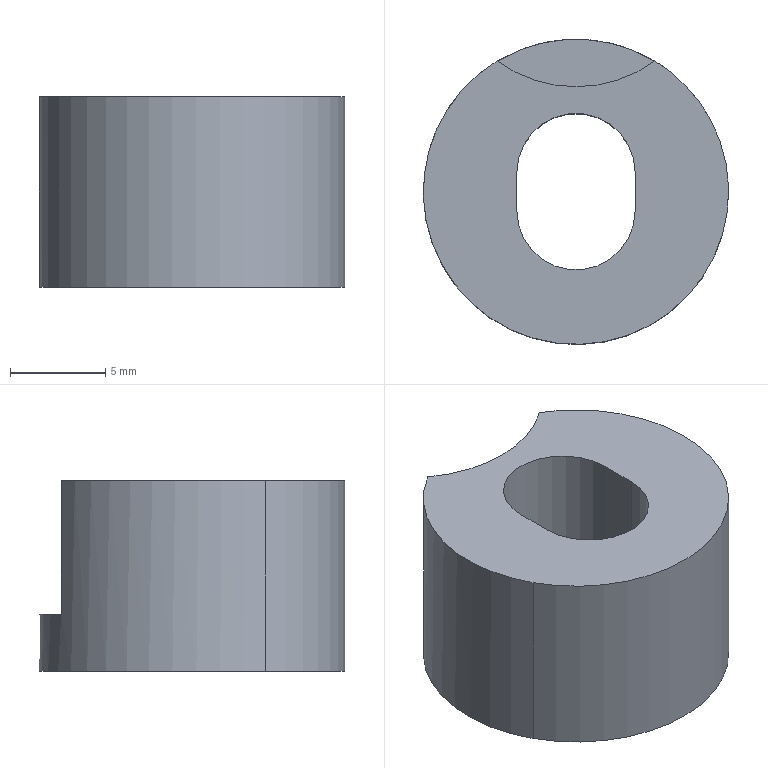Part | CATIA | 1 solid | 10 faces | box 16 x 16 x 10 mm | volume 1487 mm3 | cylinder 5 | plane 5 | commonest cylinder face diameters 6.2 x2 16 x2 14 x1
STEP:
#1=CARTESIAN_POINT('',(7.021,3.835,-10.));
#2=VERTEX_POINT('',#1);
#3=CARTESIAN_POINT('',(7.021,3.835,0.));
#4=VERTEX_POINT('',#3);
#5=CARTESIAN_POINT('',(7.021,3.835,-5.));
#6=DIRECTION('',(0.,0.,1.));
#7=VECTOR('',#6,1.);
#8=LINE('',#5,#7);
#9=EDGE_CURVE('',#2,#4,#8,.T.);
#10=ORIENTED_EDGE('',*,*,#9,.T.);
#11=CARTESIAN_POINT('',(-7.021,-3.835,0.));
#12=VERTEX_POINT('',#11);
#13=CARTESIAN_POINT('',(0.,0.,0.));
#14=DIRECTION('',(0.,0.,1.));
#15=AXIS2_PLACEMENT_3D('',#13,#14,$);
#16=CIRCLE('',#15,8.);
#17=EDGE_CURVE('',#12,#4,#16,.T.);
#18=ORIENTED_EDGE('',*,*,#17,.F.);
#19=CARTESIAN_POINT('',(-7.021,-3.835,-10.));
#20=VERTEX_POINT('',#19);
#21=CARTESIAN_POINT('',(-7.021,-3.835,-5.));
#22=DIRECTION('',(0.,0.,1.));
#23=VECTOR('',#22,1.);
#24=LINE('',#21,#23);
#25=EDGE_CURVE('',#20,#12,#24,.T.);
#26=ORIENTED_EDGE('',*,*,#25,.F.);
#27=CARTESIAN_POINT('',(0.,0.,-10.));
#28=DIRECTION('',(0.,0.,1.));
#29=AXIS2_PLACEMENT_3D('',#27,#28,$);
#30=CIRCLE('',#29,8.);
#31=EDGE_CURVE('',#20,#2,#30,.T.);
#32=ORIENTED_EDGE('',*,*,#31,.T.);
#33=EDGE_LOOP('',(#10,#18,#26,#32));
#34=FACE_OUTER_BOUND('',#33,.T.);
#35=CARTESIAN_POINT('',(0.,0.,-5.));
#36=DIRECTION('',(0.,0.,1.));
#37=DIRECTION('',(0.8776,0.4794,0.));
#38=AXIS2_PLACEMENT_3D('',#35,#36,#37);
#39=CYLINDRICAL_SURFACE('',#38,8.);
#40=ADVANCED_FACE('',(#34),#39,.T.);
#41=ORIENTED_EDGE('',*,*,#31,.F.);
#42=CARTESIAN_POINT('',(0.,0.,-10.));
#43=DIRECTION('',(0.,0.,1.));
#44=AXIS2_PLACEMENT_3D('',#42,#43,$);
#45=CIRCLE('',#44,8.);
#46=EDGE_CURVE('',#2,#20,#45,.T.);
#47=ORIENTED_EDGE('',*,*,#46,.F.);
#48=EDGE_LOOP('',(#41,#47));
#49=FACE_OUTER_BOUND('',#48,.T.);
#50=CARTESIAN_POINT('',(3.1,1.,-10.));
#51=VERTEX_POINT('',#50);
#52=CARTESIAN_POINT('',(-3.1,1.,-10.));
#53=VERTEX_POINT('',#52);
#54=CARTESIAN_POINT('',(0.,1.,-10.));
#55=DIRECTION('',(0.,0.,1.));
#56=AXIS2_PLACEMENT_3D('',#54,#55,$);
#57=CIRCLE('',#56,3.1);
#58=EDGE_CURVE('',#51,#53,#57,.T.);
#59=ORIENTED_EDGE('',*,*,#58,.T.);
#60=CARTESIAN_POINT('',(-3.1,-1.,-10.));
#61=VERTEX_POINT('',#60);
#62=CARTESIAN_POINT('',(-3.1,0.,-10.));
#63=DIRECTION('',(0.,1.,0.));
#64=VECTOR('',#63,1.);
#65=LINE('',#62,#64);
#66=EDGE_CURVE('',#61,#53,#65,.T.);
#67=ORIENTED_EDGE('',*,*,#66,.F.);
#68=CARTESIAN_POINT('',(3.1,-1.,-10.));
#69=VERTEX_POINT('',#68);
#70=CARTESIAN_POINT('',(0.,-1.,-10.));
#71=DIRECTION('',(0.,0.,1.));
#72=AXIS2_PLACEMENT_3D('',#70,#71,$);
#73=CIRCLE('',#72,3.1);
#74=EDGE_CURVE('',#61,#69,#73,.T.);
#75=ORIENTED_EDGE('',*,*,#74,.T.);
#76=CARTESIAN_POINT('',(3.1,0.,-10.));
#77=DIRECTION('',(0.,-1.,0.));
#78=VECTOR('',#77,1.);
#79=LINE('',#76,#78);
#80=EDGE_CURVE('',#51,#69,#79,.T.);
#81=ORIENTED_EDGE('',*,*,#80,.F.);
#82=EDGE_LOOP('',(#59,#67,#75,#81));
#83=FACE_BOUND('',#82,.T.);
#84=CARTESIAN_POINT('',(8.,0.,-10.));
#85=DIRECTION('',(0.,0.,1.));
#86=DIRECTION('',(1.,0.,0.));
#87=AXIS2_PLACEMENT_3D('',#84,#85,#86);
#88=PLANE('',#87);
#89=ADVANCED_FACE('',(#49,#83),#88,.F.);
#90=ORIENTED_EDGE('',*,*,#58,.F.);
#91=CARTESIAN_POINT('',(3.1,1.,0.));
#92=VERTEX_POINT('',#91);
#93=CARTESIAN_POINT('',(3.1,1.,-16.61));
#94=DIRECTION('',(0.,0.,-1.));
#95=VECTOR('',#94,1.);
#96=LINE('',#93,#95);
#97=EDGE_CURVE('',#92,#51,#96,.T.);
#98=ORIENTED_EDGE('',*,*,#97,.F.);
#99=CARTESIAN_POINT('',(-3.1,1.,0.));
#100=VERTEX_POINT('',#99);
#101=CARTESIAN_POINT('',(0.,1.,0.));
#102=DIRECTION('',(0.,0.,-1.));
#103=AXIS2_PLACEMENT_3D('',#101,#102,$);
#104=CIRCLE('',#103,3.1);
#105=EDGE_CURVE('',#100,#92,#104,.T.);
#106=ORIENTED_EDGE('',*,*,#105,.F.);
#107=CARTESIAN_POINT('',(-3.1,1.,-16.61));
#108=DIRECTION('',(0.,0.,-1.));
#109=VECTOR('',#108,1.);
#110=LINE('',#107,#109);
#111=EDGE_CURVE('',#100,#53,#110,.T.);
#112=ORIENTED_EDGE('',*,*,#111,.T.);
#113=EDGE_LOOP('',(#90,#98,#106,#112));
#114=FACE_OUTER_BOUND('',#113,.T.);
#115=CARTESIAN_POINT('',(0.,1.,-16.61));
#116=DIRECTION('',(0.,0.,-1.));
#117=DIRECTION('',(-1.,0.,0.));
#118=AXIS2_PLACEMENT_3D('',#115,#116,#117);
#119=CYLINDRICAL_SURFACE('',#118,3.1);
#120=ADVANCED_FACE('',(#114),#119,.F.);
#121=ORIENTED_EDGE('',*,*,#66,.T.);
#122=ORIENTED_EDGE('',*,*,#111,.F.);
#123=CARTESIAN_POINT('',(-3.1,-1.,0.));
#124=VERTEX_POINT('',#123);
#125=CARTESIAN_POINT('',(-3.1,0.,0.));
#126=DIRECTION('',(0.,1.,0.));
#127=VECTOR('',#126,1.);
#128=LINE('',#125,#127);
#129=EDGE_CURVE('',#124,#100,#128,.T.);
#130=ORIENTED_EDGE('',*,*,#129,.F.);
#131=CARTESIAN_POINT('',(-3.1,-1.,-5.));
#132=DIRECTION('',(0.,0.,-1.));
#133=VECTOR('',#132,1.);
#134=LINE('',#131,#133);
#135=EDGE_CURVE('',#124,#61,#134,.T.);
#136=ORIENTED_EDGE('',*,*,#135,.T.);
#137=EDGE_LOOP('',(#121,#122,#130,#136));
#138=FACE_OUTER_BOUND('',#137,.T.);
#139=CARTESIAN_POINT('',(-3.1,-1.,0.));
#140=DIRECTION('',(-1.,0.,0.));
#141=DIRECTION('',(0.,1.,0.));
#142=AXIS2_PLACEMENT_3D('',#139,#140,#141);
#143=PLANE('',#142);
#144=ADVANCED_FACE('',(#138),#143,.F.);
#145=ORIENTED_EDGE('',*,*,#80,.T.);
#146=CARTESIAN_POINT('',(3.1,-1.,0.));
#147=VERTEX_POINT('',#146);
#148=CARTESIAN_POINT('',(3.1,-1.,-5.));
#149=DIRECTION('',(0.,0.,-1.));
#150=VECTOR('',#149,1.);
#151=LINE('',#148,#150);
#152=EDGE_CURVE('',#147,#69,#151,.T.);
#153=ORIENTED_EDGE('',*,*,#152,.F.);
#154=CARTESIAN_POINT('',(3.1,0.,0.));
#155=DIRECTION('',(0.,-1.,0.));
#156=VECTOR('',#155,1.);
#157=LINE('',#154,#156);
#158=EDGE_CURVE('',#92,#147,#157,.T.);
#159=ORIENTED_EDGE('',*,*,#158,.F.);
#160=ORIENTED_EDGE('',*,*,#97,.T.);
#161=EDGE_LOOP('',(#145,#153,#159,#160));
#162=FACE_OUTER_BOUND('',#161,.T.);
#163=CARTESIAN_POINT('',(3.1,1.,0.));
#164=DIRECTION('',(1.,0.,0.));
#165=DIRECTION('',(0.,-1.,0.));
#166=AXIS2_PLACEMENT_3D('',#163,#164,#165);
#167=PLANE('',#166);
#168=ADVANCED_FACE('',(#162),#167,.F.);
#169=ORIENTED_EDGE('',*,*,#74,.F.);
#170=ORIENTED_EDGE('',*,*,#135,.F.);
#171=CARTESIAN_POINT('',(0.,-1.,0.));
#172=DIRECTION('',(0.,0.,-1.));
#173=AXIS2_PLACEMENT_3D('',#171,#172,$);
#174=CIRCLE('',#173,3.1);
#175=EDGE_CURVE('',#147,#124,#174,.T.);
#176=ORIENTED_EDGE('',*,*,#175,.F.);
#177=ORIENTED_EDGE('',*,*,#152,.T.);
#178=EDGE_LOOP('',(#169,#170,#176,#177));
#179=FACE_OUTER_BOUND('',#178,.T.);
#180=CARTESIAN_POINT('',(0.,-1.,-16.61));
#181=DIRECTION('',(0.,0.,-1.));
#182=DIRECTION('',(1.,0.,0.));
#183=AXIS2_PLACEMENT_3D('',#180,#181,#182);
#184=CYLINDRICAL_SURFACE('',#183,3.1);
#185=ADVANCED_FACE('',(#179),#184,.F.);
#186=CARTESIAN_POINT('',(-4.132,6.85,0.));
#187=VERTEX_POINT('',#186);
#188=CARTESIAN_POINT('',(0.,0.,0.));
#189=DIRECTION('',(0.,0.,1.));
#190=AXIS2_PLACEMENT_3D('',#188,#189,$);
#191=CIRCLE('',#190,8.);
#192=EDGE_CURVE('',#187,#12,#191,.T.);
#193=ORIENTED_EDGE('',*,*,#192,.T.);
#194=ORIENTED_EDGE('',*,*,#17,.T.);
#195=CARTESIAN_POINT('',(4.132,6.85,0.));
#196=VERTEX_POINT('',#195);
#197=CARTESIAN_POINT('',(0.,0.,0.));
#198=DIRECTION('',(0.,0.,1.));
#199=AXIS2_PLACEMENT_3D('',#197,#198,$);
#200=CIRCLE('',#199,8.);
#201=EDGE_CURVE('',#4,#196,#200,.T.);
#202=ORIENTED_EDGE('',*,*,#201,.T.);
#203=CARTESIAN_POINT('',(0.,12.5,0.));
#204=DIRECTION('',(0.,0.,1.));
#205=AXIS2_PLACEMENT_3D('',#203,#204,$);
#206=CIRCLE('',#205,7.);
#207=EDGE_CURVE('',#187,#196,#206,.T.);
#208=ORIENTED_EDGE('',*,*,#207,.F.);
#209=EDGE_LOOP('',(#193,#194,#202,#208));
#210=FACE_OUTER_BOUND('',#209,.T.);
#211=ORIENTED_EDGE('',*,*,#105,.T.);
#212=ORIENTED_EDGE('',*,*,#158,.T.);
#213=ORIENTED_EDGE('',*,*,#175,.T.);
#214=ORIENTED_EDGE('',*,*,#129,.T.);
#215=EDGE_LOOP('',(#211,#212,#213,#214));
#216=FACE_BOUND('',#215,.T.);
#217=CARTESIAN_POINT('',(0.,0.,0.));
#218=DIRECTION('',(0.,0.,1.));
#219=DIRECTION('',(1.,0.,0.));
#220=AXIS2_PLACEMENT_3D('',#217,#218,#219);
#221=PLANE('',#220);
#222=ADVANCED_FACE('',(#210,#216),#221,.T.);
#223=ORIENTED_EDGE('',*,*,#201,.F.);
#224=ORIENTED_EDGE('',*,*,#9,.F.);
#225=ORIENTED_EDGE('',*,*,#46,.T.);
#226=ORIENTED_EDGE('',*,*,#25,.T.);
#227=ORIENTED_EDGE('',*,*,#192,.F.);
#228=CARTESIAN_POINT('',(-4.132,6.85,-7.));
#229=VERTEX_POINT('',#228);
#230=CARTESIAN_POINT('',(-4.132,6.85,-5.));
#231=DIRECTION('',(0.,0.,1.));
#232=VECTOR('',#231,1.);
#233=LINE('',#230,#232);
#234=EDGE_CURVE('',#229,#187,#233,.T.);
#235=ORIENTED_EDGE('',*,*,#234,.F.);
#236=CARTESIAN_POINT('',(4.132,6.85,-7.));
#237=VERTEX_POINT('',#236);
#238=CARTESIAN_POINT('',(0.,0.,-7.));
#239=DIRECTION('',(0.,0.,1.));
#240=AXIS2_PLACEMENT_3D('',#238,#239,$);
#241=CIRCLE('',#240,8.);
#242=EDGE_CURVE('',#237,#229,#241,.T.);
#243=ORIENTED_EDGE('',*,*,#242,.F.);
#244=CARTESIAN_POINT('',(4.132,6.85,-5.));
#245=DIRECTION('',(0.,0.,1.));
#246=VECTOR('',#245,1.);
#247=LINE('',#244,#246);
#248=EDGE_CURVE('',#237,#196,#247,.T.);
#249=ORIENTED_EDGE('',*,*,#248,.T.);
#250=EDGE_LOOP('',(#223,#224,#225,#226,#227,#235,#243,#249));
#251=FACE_OUTER_BOUND('',#250,.T.);
#252=ADVANCED_FACE('',(#251),#39,.T.);
#253=CARTESIAN_POINT('',(0.,12.5,-7.));
#254=DIRECTION('',(0.,0.,1.));
#255=AXIS2_PLACEMENT_3D('',#253,#254,$);
#256=CIRCLE('',#255,7.);
#257=EDGE_CURVE('',#229,#237,#256,.T.);
#258=ORIENTED_EDGE('',*,*,#257,.T.);
#259=ORIENTED_EDGE('',*,*,#242,.T.);
#260=EDGE_LOOP('',(#258,#259));
#261=FACE_OUTER_BOUND('',#260,.T.);
#262=CARTESIAN_POINT('',(0.,0.,-7.));
#263=DIRECTION('',(0.,0.,1.));
#264=DIRECTION('',(1.,0.,0.));
#265=AXIS2_PLACEMENT_3D('',#262,#263,#264);
#266=PLANE('',#265);
#267=ADVANCED_FACE('',(#261),#266,.T.);
#268=ORIENTED_EDGE('',*,*,#207,.T.);
#269=ORIENTED_EDGE('',*,*,#248,.F.);
#270=ORIENTED_EDGE('',*,*,#257,.F.);
#271=ORIENTED_EDGE('',*,*,#234,.T.);
#272=EDGE_LOOP('',(#268,#269,#270,#271));
#273=FACE_OUTER_BOUND('',#272,.T.);
#274=CARTESIAN_POINT('',(0.,12.5,-4.11));
#275=DIRECTION('',(0.,0.,1.));
#276=DIRECTION('',(1.,0.,0.));
#277=AXIS2_PLACEMENT_3D('',#274,#275,#276);
#278=CYLINDRICAL_SURFACE('',#277,7.);
#279=ADVANCED_FACE('',(#273),#278,.F.);
#280=CLOSED_SHELL('',(#40,#89,#120,#144,#168,#185,#222,#252,#267,#279));
#281=MANIFOLD_SOLID_BREP('',#280);
#282=(LENGTH_UNIT()NAMED_UNIT(*)SI_UNIT(.MILLI.,.METRE.));
#283=UNCERTAINTY_MEASURE_WITH_UNIT(LENGTH_MEASURE(0.005),#282,'','');
#284=(NAMED_UNIT(*)PLANE_ANGLE_UNIT()SI_UNIT($,.RADIAN.));
#285=(NAMED_UNIT(*)SI_UNIT($,.STERADIAN.)SOLID_ANGLE_UNIT());
#286=(GEOMETRIC_REPRESENTATION_CONTEXT(3)GLOBAL_UNCERTAINTY_ASSIGNED_CONTEXT((#283))GLOBAL_UNIT_ASSIGNED_CONTEXT((#282,#284,#285))REPRESENTATION_CONTEXT('',''));
#287=ADVANCED_BREP_SHAPE_REPRESENTATION('',(#281),#286);